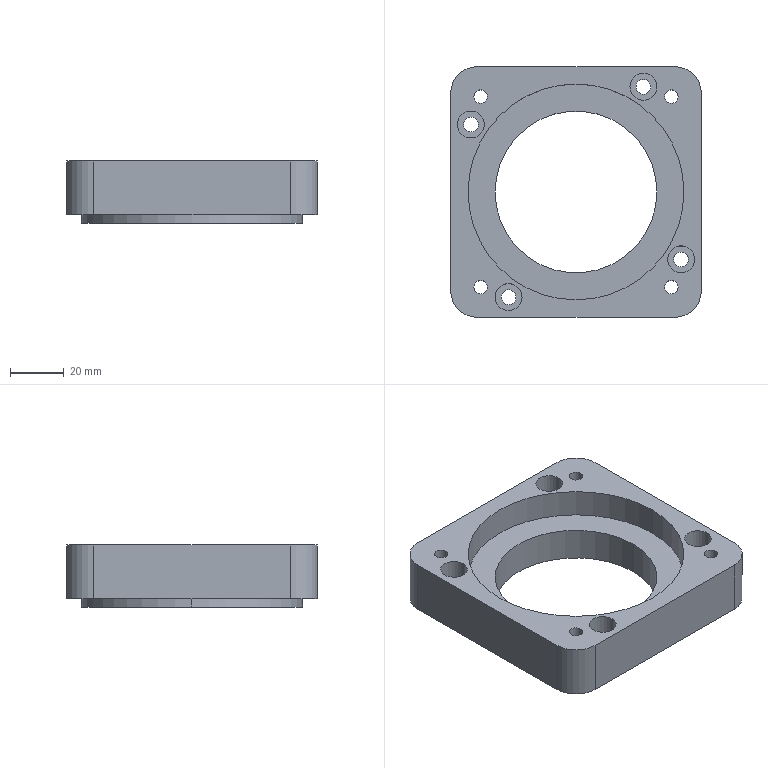Part | SolidWorks | features HoleWzd 3, CirPattern 2, ICE 2, Extrusion 1, Fillet 1 | 1 solid | 46 faces | box 93 x 93 x 23 mm | volume 93388 mm3 | cylinder 34 | plane 12 | commonest cylinder face diameters 5 x8 5.5 x8 10 x8 20 x4 60 x2 80 x2
STEP:
#1=CARTESIAN_POINT('',(-44.,25.,10.3));
#2=VERTEX_POINT('',#1);
#3=CARTESIAN_POINT('',(-34.,25.,10.3));
#4=VERTEX_POINT('',#3);
#5=CARTESIAN_POINT('',(-39.,25.,10.3));
#6=DIRECTION('',(0.,0.,1.));
#7=DIRECTION('',(1.,0.,0.));
#8=AXIS2_PLACEMENT_3D('',#5,#6,#7);
#9=CIRCLE('',#8,5.);
#10=EDGE_CURVE('',#2,#4,#9,.T.);
#11=ORIENTED_EDGE('',*,*,#10,.F.);
#12=CARTESIAN_POINT('',(-44.,25.,20.));
#13=VERTEX_POINT('',#12);
#14=CARTESIAN_POINT('',(-44.,25.,20.));
#15=DIRECTION('',(0.,0.,1.));
#16=VECTOR('',#15,1000.);
#17=LINE('',#14,#16);
#18=EDGE_CURVE('',#2,#13,#17,.T.);
#19=ORIENTED_EDGE('',*,*,#18,.T.);
#20=CARTESIAN_POINT('',(-34.,25.,20.));
#21=VERTEX_POINT('',#20);
#22=CARTESIAN_POINT('',(-39.,25.,20.));
#23=DIRECTION('',(0.,0.,1.));
#24=DIRECTION('',(1.,0.,0.));
#25=AXIS2_PLACEMENT_3D('',#22,#23,#24);
#26=CIRCLE('',#25,5.);
#27=EDGE_CURVE('',#13,#21,#26,.T.);
#28=ORIENTED_EDGE('',*,*,#27,.T.);
#29=CARTESIAN_POINT('',(-34.,25.,20.));
#30=DIRECTION('',(0.,0.,1.));
#31=VECTOR('',#30,1000.);
#32=LINE('',#29,#31);
#33=EDGE_CURVE('',#4,#21,#32,.T.);
#34=ORIENTED_EDGE('',*,*,#33,.F.);
#35=EDGE_LOOP('',(#11,#19,#28,#34));
#36=FACE_OUTER_BOUND('',#35,.T.);
#37=CARTESIAN_POINT('',(-39.,25.,20.));
#38=DIRECTION('',(0.,0.,1.));
#39=DIRECTION('',(1.,0.,0.));
#40=AXIS2_PLACEMENT_3D('',#37,#38,#39);
#41=CYLINDRICAL_SURFACE('',#40,5.);
#42=ADVANCED_FACE('',(#36),#41,.F.);
#43=CARTESIAN_POINT('',(-36.25,25.,0.));
#44=VERTEX_POINT('',#43);
#45=CARTESIAN_POINT('',(-41.75,25.,0.));
#46=VERTEX_POINT('',#45);
#47=CARTESIAN_POINT('',(-39.,25.,0.));
#48=DIRECTION('',(0.,0.,-1.));
#49=DIRECTION('',(-1.,0.,0.));
#50=AXIS2_PLACEMENT_3D('',#47,#48,#49);
#51=CIRCLE('',#50,2.75);
#52=EDGE_CURVE('',#44,#46,#51,.T.);
#53=ORIENTED_EDGE('',*,*,#52,.T.);
#54=CARTESIAN_POINT('',(-41.75,25.,10.3));
#55=VERTEX_POINT('',#54);
#56=CARTESIAN_POINT('',(-41.75,25.,20.));
#57=DIRECTION('',(0.,0.,1.));
#58=VECTOR('',#57,1000.);
#59=LINE('',#56,#58);
#60=EDGE_CURVE('',#46,#55,#59,.T.);
#61=ORIENTED_EDGE('',*,*,#60,.T.);
#62=CARTESIAN_POINT('',(-36.25,25.,10.3));
#63=VERTEX_POINT('',#62);
#64=CARTESIAN_POINT('',(-39.,25.,10.3));
#65=DIRECTION('',(0.,0.,1.));
#66=DIRECTION('',(1.,0.,0.));
#67=AXIS2_PLACEMENT_3D('',#64,#65,#66);
#68=CIRCLE('',#67,2.75);
#69=EDGE_CURVE('',#55,#63,#68,.T.);
#70=ORIENTED_EDGE('',*,*,#69,.T.);
#71=CARTESIAN_POINT('',(-36.25,25.,20.));
#72=DIRECTION('',(0.,0.,1.));
#73=VECTOR('',#72,1000.);
#74=LINE('',#71,#73);
#75=EDGE_CURVE('',#44,#63,#74,.T.);
#76=ORIENTED_EDGE('',*,*,#75,.F.);
#77=EDGE_LOOP('',(#53,#61,#70,#76));
#78=FACE_OUTER_BOUND('',#77,.T.);
#79=CARTESIAN_POINT('',(-39.,25.,20.));
#80=DIRECTION('',(0.,0.,1.));
#81=DIRECTION('',(1.,0.,0.));
#82=AXIS2_PLACEMENT_3D('',#79,#80,#81);
#83=CYLINDRICAL_SURFACE('',#82,2.75);
#84=ADVANCED_FACE('',(#78),#83,.F.);
#85=CARTESIAN_POINT('',(20.,39.,10.3));
#86=VERTEX_POINT('',#85);
#87=CARTESIAN_POINT('',(30.,39.,10.3));
#88=VERTEX_POINT('',#87);
#89=CARTESIAN_POINT('',(25.,39.,10.3));
#90=DIRECTION('',(0.,0.,1.));
#91=DIRECTION('',(1.,0.,0.));
#92=AXIS2_PLACEMENT_3D('',#89,#90,#91);
#93=CIRCLE('',#92,5.);
#94=EDGE_CURVE('',#86,#88,#93,.T.);
#95=ORIENTED_EDGE('',*,*,#94,.F.);
#96=CARTESIAN_POINT('',(20.,39.,20.));
#97=VERTEX_POINT('',#96);
#98=CARTESIAN_POINT('',(20.,39.,20.));
#99=DIRECTION('',(0.,0.,1.));
#100=VECTOR('',#99,1000.);
#101=LINE('',#98,#100);
#102=EDGE_CURVE('',#86,#97,#101,.T.);
#103=ORIENTED_EDGE('',*,*,#102,.T.);
#104=CARTESIAN_POINT('',(30.,39.,20.));
#105=VERTEX_POINT('',#104);
#106=CARTESIAN_POINT('',(25.,39.,20.));
#107=DIRECTION('',(0.,0.,1.));
#108=DIRECTION('',(1.,0.,0.));
#109=AXIS2_PLACEMENT_3D('',#106,#107,#108);
#110=CIRCLE('',#109,5.);
#111=EDGE_CURVE('',#97,#105,#110,.T.);
#112=ORIENTED_EDGE('',*,*,#111,.T.);
#113=CARTESIAN_POINT('',(30.,39.,20.));
#114=DIRECTION('',(0.,0.,1.));
#115=VECTOR('',#114,1000.);
#116=LINE('',#113,#115);
#117=EDGE_CURVE('',#88,#105,#116,.T.);
#118=ORIENTED_EDGE('',*,*,#117,.F.);
#119=EDGE_LOOP('',(#95,#103,#112,#118));
#120=FACE_OUTER_BOUND('',#119,.T.);
#121=CARTESIAN_POINT('',(25.,39.,20.));
#122=DIRECTION('',(0.,0.,1.));
#123=DIRECTION('',(1.,0.,0.));
#124=AXIS2_PLACEMENT_3D('',#121,#122,#123);
#125=CYLINDRICAL_SURFACE('',#124,5.);
#126=ADVANCED_FACE('',(#120),#125,.F.);
#127=CARTESIAN_POINT('',(27.75,39.,0.));
#128=VERTEX_POINT('',#127);
#129=CARTESIAN_POINT('',(22.25,39.,0.));
#130=VERTEX_POINT('',#129);
#131=CARTESIAN_POINT('',(25.,39.,0.));
#132=DIRECTION('',(0.,0.,-1.));
#133=DIRECTION('',(-1.,0.,0.));
#134=AXIS2_PLACEMENT_3D('',#131,#132,#133);
#135=CIRCLE('',#134,2.75);
#136=EDGE_CURVE('',#128,#130,#135,.T.);
#137=ORIENTED_EDGE('',*,*,#136,.T.);
#138=CARTESIAN_POINT('',(22.25,39.,10.3));
#139=VERTEX_POINT('',#138);
#140=CARTESIAN_POINT('',(22.25,39.,20.));
#141=DIRECTION('',(0.,0.,1.));
#142=VECTOR('',#141,1000.);
#143=LINE('',#140,#142);
#144=EDGE_CURVE('',#130,#139,#143,.T.);
#145=ORIENTED_EDGE('',*,*,#144,.T.);
#146=CARTESIAN_POINT('',(27.75,39.,10.3));
#147=VERTEX_POINT('',#146);
#148=CARTESIAN_POINT('',(25.,39.,10.3));
#149=DIRECTION('',(0.,0.,1.));
#150=DIRECTION('',(1.,0.,0.));
#151=AXIS2_PLACEMENT_3D('',#148,#149,#150);
#152=CIRCLE('',#151,2.75);
#153=EDGE_CURVE('',#139,#147,#152,.T.);
#154=ORIENTED_EDGE('',*,*,#153,.T.);
#155=CARTESIAN_POINT('',(27.75,39.,20.));
#156=DIRECTION('',(0.,0.,1.));
#157=VECTOR('',#156,1000.);
#158=LINE('',#155,#157);
#159=EDGE_CURVE('',#128,#147,#158,.T.);
#160=ORIENTED_EDGE('',*,*,#159,.F.);
#161=EDGE_LOOP('',(#137,#145,#154,#160));
#162=FACE_OUTER_BOUND('',#161,.T.);
#163=CARTESIAN_POINT('',(25.,39.,20.));
#164=DIRECTION('',(0.,0.,1.));
#165=DIRECTION('',(1.,0.,0.));
#166=AXIS2_PLACEMENT_3D('',#163,#164,#165);
#167=CYLINDRICAL_SURFACE('',#166,2.75);
#168=ADVANCED_FACE('',(#162),#167,.F.);
#169=CARTESIAN_POINT('',(34.,-25.,10.3));
#170=VERTEX_POINT('',#169);
#171=CARTESIAN_POINT('',(44.,-25.,10.3));
#172=VERTEX_POINT('',#171);
#173=CARTESIAN_POINT('',(39.,-25.,10.3));
#174=DIRECTION('',(0.,0.,1.));
#175=DIRECTION('',(1.,0.,0.));
#176=AXIS2_PLACEMENT_3D('',#173,#174,#175);
#177=CIRCLE('',#176,5.);
#178=EDGE_CURVE('',#170,#172,#177,.T.);
#179=ORIENTED_EDGE('',*,*,#178,.F.);
#180=CARTESIAN_POINT('',(34.,-25.,20.));
#181=VERTEX_POINT('',#180);
#182=CARTESIAN_POINT('',(34.,-25.,20.));
#183=DIRECTION('',(0.,0.,1.));
#184=VECTOR('',#183,1000.);
#185=LINE('',#182,#184);
#186=EDGE_CURVE('',#170,#181,#185,.T.);
#187=ORIENTED_EDGE('',*,*,#186,.T.);
#188=CARTESIAN_POINT('',(44.,-25.,20.));
#189=VERTEX_POINT('',#188);
#190=CARTESIAN_POINT('',(39.,-25.,20.));
#191=DIRECTION('',(0.,0.,1.));
#192=DIRECTION('',(1.,0.,0.));
#193=AXIS2_PLACEMENT_3D('',#190,#191,#192);
#194=CIRCLE('',#193,5.);
#195=EDGE_CURVE('',#181,#189,#194,.T.);
#196=ORIENTED_EDGE('',*,*,#195,.T.);
#197=CARTESIAN_POINT('',(44.,-25.,20.));
#198=DIRECTION('',(0.,0.,1.));
#199=VECTOR('',#198,1000.);
#200=LINE('',#197,#199);
#201=EDGE_CURVE('',#172,#189,#200,.T.);
#202=ORIENTED_EDGE('',*,*,#201,.F.);
#203=EDGE_LOOP('',(#179,#187,#196,#202));
#204=FACE_OUTER_BOUND('',#203,.T.);
#205=CARTESIAN_POINT('',(39.,-25.,20.));
#206=DIRECTION('',(0.,0.,1.));
#207=DIRECTION('',(1.,0.,0.));
#208=AXIS2_PLACEMENT_3D('',#205,#206,#207);
#209=CYLINDRICAL_SURFACE('',#208,5.);
#210=ADVANCED_FACE('',(#204),#209,.F.);
#211=CARTESIAN_POINT('',(41.75,-25.,0.));
#212=VERTEX_POINT('',#211);
#213=CARTESIAN_POINT('',(36.25,-25.,0.));
#214=VERTEX_POINT('',#213);
#215=CARTESIAN_POINT('',(39.,-25.,0.));
#216=DIRECTION('',(0.,0.,-1.));
#217=DIRECTION('',(-1.,0.,0.));
#218=AXIS2_PLACEMENT_3D('',#215,#216,#217);
#219=CIRCLE('',#218,2.75);
#220=EDGE_CURVE('',#212,#214,#219,.T.);
#221=ORIENTED_EDGE('',*,*,#220,.T.);
#222=CARTESIAN_POINT('',(36.25,-25.,10.3));
#223=VERTEX_POINT('',#222);
#224=CARTESIAN_POINT('',(36.25,-25.,20.));
#225=DIRECTION('',(0.,0.,1.));
#226=VECTOR('',#225,1000.);
#227=LINE('',#224,#226);
#228=EDGE_CURVE('',#214,#223,#227,.T.);
#229=ORIENTED_EDGE('',*,*,#228,.T.);
#230=CARTESIAN_POINT('',(41.75,-25.,10.3));
#231=VERTEX_POINT('',#230);
#232=CARTESIAN_POINT('',(39.,-25.,10.3));
#233=DIRECTION('',(0.,0.,1.));
#234=DIRECTION('',(1.,0.,0.));
#235=AXIS2_PLACEMENT_3D('',#232,#233,#234);
#236=CIRCLE('',#235,2.75);
#237=EDGE_CURVE('',#223,#231,#236,.T.);
#238=ORIENTED_EDGE('',*,*,#237,.T.);
#239=CARTESIAN_POINT('',(41.75,-25.,20.));
#240=DIRECTION('',(0.,0.,1.));
#241=VECTOR('',#240,1000.);
#242=LINE('',#239,#241);
#243=EDGE_CURVE('',#212,#231,#242,.T.);
#244=ORIENTED_EDGE('',*,*,#243,.F.);
#245=EDGE_LOOP('',(#221,#229,#238,#244));
#246=FACE_OUTER_BOUND('',#245,.T.);
#247=CARTESIAN_POINT('',(39.,-25.,20.));
#248=DIRECTION('',(0.,0.,1.));
#249=DIRECTION('',(1.,0.,0.));
#250=AXIS2_PLACEMENT_3D('',#247,#248,#249);
#251=CYLINDRICAL_SURFACE('',#250,2.75);
#252=ADVANCED_FACE('',(#246),#251,.F.);
#253=CARTESIAN_POINT('',(-30.,-39.,10.3));
#254=VERTEX_POINT('',#253);
#255=CARTESIAN_POINT('',(-20.,-39.,10.3));
#256=VERTEX_POINT('',#255);
#257=CARTESIAN_POINT('',(-25.,-39.,10.3));
#258=DIRECTION('',(0.,0.,1.));
#259=DIRECTION('',(1.,0.,0.));
#260=AXIS2_PLACEMENT_3D('',#257,#258,#259);
#261=CIRCLE('',#260,5.);
#262=EDGE_CURVE('',#254,#256,#261,.T.);
#263=ORIENTED_EDGE('',*,*,#262,.F.);
#264=CARTESIAN_POINT('',(-30.,-39.,20.));
#265=VERTEX_POINT('',#264);
#266=CARTESIAN_POINT('',(-30.,-39.,20.));
#267=DIRECTION('',(0.,0.,1.));
#268=VECTOR('',#267,1000.);
#269=LINE('',#266,#268);
#270=EDGE_CURVE('',#254,#265,#269,.T.);
#271=ORIENTED_EDGE('',*,*,#270,.T.);
#272=CARTESIAN_POINT('',(-20.,-39.,20.));
#273=VERTEX_POINT('',#272);
#274=CARTESIAN_POINT('',(-25.,-39.,20.));
#275=DIRECTION('',(0.,0.,1.));
#276=DIRECTION('',(1.,0.,0.));
#277=AXIS2_PLACEMENT_3D('',#274,#275,#276);
#278=CIRCLE('',#277,5.);
#279=EDGE_CURVE('',#265,#273,#278,.T.);
#280=ORIENTED_EDGE('',*,*,#279,.T.);
#281=CARTESIAN_POINT('',(-20.,-39.,20.));
#282=DIRECTION('',(0.,0.,1.));
#283=VECTOR('',#282,1000.);
#284=LINE('',#281,#283);
#285=EDGE_CURVE('',#256,#273,#284,.T.);
#286=ORIENTED_EDGE('',*,*,#285,.F.);
#287=EDGE_LOOP('',(#263,#271,#280,#286));
#288=FACE_OUTER_BOUND('',#287,.T.);
#289=CARTESIAN_POINT('',(-25.,-39.,20.));
#290=DIRECTION('',(0.,0.,1.));
#291=DIRECTION('',(1.,0.,0.));
#292=AXIS2_PLACEMENT_3D('',#289,#290,#291);
#293=CYLINDRICAL_SURFACE('',#292,5.);
#294=ADVANCED_FACE('',(#288),#293,.F.);
#295=CARTESIAN_POINT('',(-22.25,-39.,0.));
#296=VERTEX_POINT('',#295);
#297=CARTESIAN_POINT('',(-27.75,-39.,0.));
#298=VERTEX_POINT('',#297);
#299=CARTESIAN_POINT('',(-25.,-39.,0.));
#300=DIRECTION('',(0.,0.,-1.));
#301=DIRECTION('',(-1.,0.,0.));
#302=AXIS2_PLACEMENT_3D('',#299,#300,#301);
#303=CIRCLE('',#302,2.75);
#304=EDGE_CURVE('',#296,#298,#303,.T.);
#305=ORIENTED_EDGE('',*,*,#304,.T.);
#306=CARTESIAN_POINT('',(-27.75,-39.,10.3));
#307=VERTEX_POINT('',#306);
#308=CARTESIAN_POINT('',(-27.75,-39.,20.));
#309=DIRECTION('',(0.,0.,1.));
#310=VECTOR('',#309,1000.);
#311=LINE('',#308,#310);
#312=EDGE_CURVE('',#298,#307,#311,.T.);
#313=ORIENTED_EDGE('',*,*,#312,.T.);
#314=CARTESIAN_POINT('',(-22.25,-39.,10.3));
#315=VERTEX_POINT('',#314);
#316=CARTESIAN_POINT('',(-25.,-39.,10.3));
#317=DIRECTION('',(0.,0.,1.));
#318=DIRECTION('',(1.,0.,0.));
#319=AXIS2_PLACEMENT_3D('',#316,#317,#318);
#320=CIRCLE('',#319,2.75);
#321=EDGE_CURVE('',#307,#315,#320,.T.);
#322=ORIENTED_EDGE('',*,*,#321,.T.);
#323=CARTESIAN_POINT('',(-22.25,-39.,20.));
#324=DIRECTION('',(0.,0.,1.));
#325=VECTOR('',#324,1000.);
#326=LINE('',#323,#325);
#327=EDGE_CURVE('',#296,#315,#326,.T.);
#328=ORIENTED_EDGE('',*,*,#327,.F.);
#329=EDGE_LOOP('',(#305,#313,#322,#328));
#330=FACE_OUTER_BOUND('',#329,.T.);
#331=CARTESIAN_POINT('',(-25.,-39.,20.));
#332=DIRECTION('',(0.,0.,1.));
#333=DIRECTION('',(1.,0.,0.));
#334=AXIS2_PLACEMENT_3D('',#331,#332,#333);
#335=CYLINDRICAL_SURFACE('',#334,2.75);
#336=ADVANCED_FACE('',(#330),#335,.F.);
#337=CARTESIAN_POINT('',(-32.855,35.355,0.));
#338=VERTEX_POINT('',#337);
#339=CARTESIAN_POINT('',(-37.855,35.355,0.));
#340=VERTEX_POINT('',#339);
#341=CARTESIAN_POINT('',(-35.355,35.355,0.));
#342=DIRECTION('',(0.,0.,-1.));
#343=DIRECTION('',(-1.,0.,0.));
#344=AXIS2_PLACEMENT_3D('',#341,#342,#343);
#345=CIRCLE('',#344,2.5);
#346=EDGE_CURVE('',#338,#340,#345,.T.);
#347=ORIENTED_EDGE('',*,*,#346,.T.);
#348=CARTESIAN_POINT('',(-37.855,35.355,20.));
#349=VERTEX_POINT('',#348);
#350=CARTESIAN_POINT('',(-37.855,35.355,20.));
#351=DIRECTION('',(0.,0.,1.));
#352=VECTOR('',#351,1000.);
#353=LINE('',#350,#352);
#354=EDGE_CURVE('',#340,#349,#353,.T.);
#355=ORIENTED_EDGE('',*,*,#354,.T.);
#356=CARTESIAN_POINT('',(-32.855,35.355,20.));
#357=VERTEX_POINT('',#356);
#358=CARTESIAN_POINT('',(-35.355,35.355,20.));
#359=DIRECTION('',(0.,0.,1.));
#360=DIRECTION('',(1.,0.,0.));
#361=AXIS2_PLACEMENT_3D('',#358,#359,#360);
#362=CIRCLE('',#361,2.5);
#363=EDGE_CURVE('',#349,#357,#362,.T.);
#364=ORIENTED_EDGE('',*,*,#363,.T.);
#365=CARTESIAN_POINT('',(-32.855,35.355,20.));
#366=DIRECTION('',(0.,0.,1.));
#367=VECTOR('',#366,1000.);
#368=LINE('',#365,#367);
#369=EDGE_CURVE('',#338,#357,#368,.T.);
#370=ORIENTED_EDGE('',*,*,#369,.F.);
#371=EDGE_LOOP('',(#347,#355,#364,#370));
#372=FACE_OUTER_BOUND('',#371,.T.);
#373=CARTESIAN_POINT('',(-35.355,35.355,20.));
#374=DIRECTION('',(0.,0.,1.));
#375=DIRECTION('',(1.,0.,0.));
#376=AXIS2_PLACEMENT_3D('',#373,#374,#375);
#377=CYLINDRICAL_SURFACE('',#376,2.5);
#378=ADVANCED_FACE('',(#372),#377,.F.);
#379=CARTESIAN_POINT('',(37.855,35.355,0.));
#380=VERTEX_POINT('',#379);
#381=CARTESIAN_POINT('',(32.855,35.355,0.));
#382=VERTEX_POINT('',#381);
#383=CARTESIAN_POINT('',(35.355,35.355,0.));
#384=DIRECTION('',(0.,0.,-1.));
#385=DIRECTION('',(-1.,0.,0.));
#386=AXIS2_PLACEMENT_3D('',#383,#384,#385);
#387=CIRCLE('',#386,2.5);
#388=EDGE_CURVE('',#380,#382,#387,.T.);
#389=ORIENTED_EDGE('',*,*,#388,.T.);
#390=CARTESIAN_POINT('',(32.855,35.355,20.));
#391=VERTEX_POINT('',#390);
#392=CARTESIAN_POINT('',(32.855,35.355,20.));
#393=DIRECTION('',(0.,0.,1.));
#394=VECTOR('',#393,1000.);
#395=LINE('',#392,#394);
#396=EDGE_CURVE('',#382,#391,#395,.T.);
#397=ORIENTED_EDGE('',*,*,#396,.T.);
#398=CARTESIAN_POINT('',(37.855,35.355,20.));
#399=VERTEX_POINT('',#398);
#400=CARTESIAN_POINT('',(35.355,35.355,20.));
#401=DIRECTION('',(0.,0.,1.));
#402=DIRECTION('',(1.,0.,0.));
#403=AXIS2_PLACEMENT_3D('',#400,#401,#402);
#404=CIRCLE('',#403,2.5);
#405=EDGE_CURVE('',#391,#399,#404,.T.);
#406=ORIENTED_EDGE('',*,*,#405,.T.);
#407=CARTESIAN_POINT('',(37.855,35.355,20.));
#408=DIRECTION('',(0.,0.,1.));
#409=VECTOR('',#408,1000.);
#410=LINE('',#407,#409);
#411=EDGE_CURVE('',#380,#399,#410,.T.);
#412=ORIENTED_EDGE('',*,*,#411,.F.);
#413=EDGE_LOOP('',(#389,#397,#406,#412));
#414=FACE_OUTER_BOUND('',#413,.T.);
#415=CARTESIAN_POINT('',(35.355,35.355,20.));
#416=DIRECTION('',(0.,0.,1.));
#417=DIRECTION('',(1.,0.,0.));
#418=AXIS2_PLACEMENT_3D('',#415,#416,#417);
#419=CYLINDRICAL_SURFACE('',#418,2.5);
#420=ADVANCED_FACE('',(#414),#419,.F.);
#421=CARTESIAN_POINT('',(37.855,-35.355,0.));
#422=VERTEX_POINT('',#421);
#423=CARTESIAN_POINT('',(32.855,-35.355,0.));
#424=VERTEX_POINT('',#423);
#425=CARTESIAN_POINT('',(35.355,-35.355,0.));
#426=DIRECTION('',(0.,0.,-1.));
#427=DIRECTION('',(-1.,0.,0.));
#428=AXIS2_PLACEMENT_3D('',#425,#426,#427);
#429=CIRCLE('',#428,2.5);
#430=EDGE_CURVE('',#422,#424,#429,.T.);
#431=ORIENTED_EDGE('',*,*,#430,.T.);
#432=CARTESIAN_POINT('',(32.855,-35.355,20.));
#433=VERTEX_POINT('',#432);
#434=CARTESIAN_POINT('',(32.855,-35.355,20.));
#435=DIRECTION('',(0.,0.,1.));
#436=VECTOR('',#435,1000.);
#437=LINE('',#434,#436);
#438=EDGE_CURVE('',#424,#433,#437,.T.);
#439=ORIENTED_EDGE('',*,*,#438,.T.);
#440=CARTESIAN_POINT('',(37.855,-35.355,20.));
#441=VERTEX_POINT('',#440);
#442=CARTESIAN_POINT('',(35.355,-35.355,20.));
#443=DIRECTION('',(0.,0.,1.));
#444=DIRECTION('',(1.,0.,0.));
#445=AXIS2_PLACEMENT_3D('',#442,#443,#444);
#446=CIRCLE('',#445,2.5);
#447=EDGE_CURVE('',#433,#441,#446,.T.);
#448=ORIENTED_EDGE('',*,*,#447,.T.);
#449=CARTESIAN_POINT('',(37.855,-35.355,20.));
#450=DIRECTION('',(0.,0.,1.));
#451=VECTOR('',#450,1000.);
#452=LINE('',#449,#451);
#453=EDGE_CURVE('',#422,#441,#452,.T.);
#454=ORIENTED_EDGE('',*,*,#453,.F.);
#455=EDGE_LOOP('',(#431,#439,#448,#454));
#456=FACE_OUTER_BOUND('',#455,.T.);
#457=CARTESIAN_POINT('',(35.355,-35.355,20.));
#458=DIRECTION('',(0.,0.,1.));
#459=DIRECTION('',(1.,0.,0.));
#460=AXIS2_PLACEMENT_3D('',#457,#458,#459);
#461=CYLINDRICAL_SURFACE('',#460,2.5);
#462=ADVANCED_FACE('',(#456),#461,.F.);
#463=CARTESIAN_POINT('',(-32.855,-35.355,0.));
#464=VERTEX_POINT('',#463);
#465=CARTESIAN_POINT('',(-37.855,-35.355,0.));
#466=VERTEX_POINT('',#465);
#467=CARTESIAN_POINT('',(-35.355,-35.355,0.));
#468=DIRECTION('',(0.,0.,-1.));
#469=DIRECTION('',(-1.,0.,0.));
#470=AXIS2_PLACEMENT_3D('',#467,#468,#469);
#471=CIRCLE('',#470,2.5);
#472=EDGE_CURVE('',#464,#466,#471,.T.);
#473=ORIENTED_EDGE('',*,*,#472,.T.);
#474=CARTESIAN_POINT('',(-37.855,-35.355,20.));
#475=VERTEX_POINT('',#474);
#476=CARTESIAN_POINT('',(-37.855,-35.355,20.));
#477=DIRECTION('',(0.,0.,1.));
#478=VECTOR('',#477,1000.);
#479=LINE('',#476,#478);
#480=EDGE_CURVE('',#466,#475,#479,.T.);
#481=ORIENTED_EDGE('',*,*,#480,.T.);
#482=CARTESIAN_POINT('',(-32.855,-35.355,20.));
#483=VERTEX_POINT('',#482);
#484=CARTESIAN_POINT('',(-35.355,-35.355,20.));
#485=DIRECTION('',(0.,0.,1.));
#486=DIRECTION('',(1.,0.,0.));
#487=AXIS2_PLACEMENT_3D('',#484,#485,#486);
#488=CIRCLE('',#487,2.5);
#489=EDGE_CURVE('',#475,#483,#488,.T.);
#490=ORIENTED_EDGE('',*,*,#489,.T.);
#491=CARTESIAN_POINT('',(-32.855,-35.355,20.));
#492=DIRECTION('',(0.,0.,1.));
#493=VECTOR('',#492,1000.);
#494=LINE('',#491,#493);
#495=EDGE_CURVE('',#464,#483,#494,.T.);
#496=ORIENTED_EDGE('',*,*,#495,.F.);
#497=EDGE_LOOP('',(#473,#481,#490,#496));
#498=FACE_OUTER_BOUND('',#497,.T.);
#499=CARTESIAN_POINT('',(-35.355,-35.355,20.));
#500=DIRECTION('',(0.,0.,1.));
#501=DIRECTION('',(1.,0.,0.));
#502=AXIS2_PLACEMENT_3D('',#499,#500,#501);
#503=CYLINDRICAL_SURFACE('',#502,2.5);
#504=ADVANCED_FACE('',(#498),#503,.F.);
#505=CARTESIAN_POINT('',(-40.,0.,9.5));
#506=VERTEX_POINT('',#505);
#507=CARTESIAN_POINT('',(40.,0.,9.5));
#508=VERTEX_POINT('',#507);
#509=CARTESIAN_POINT('',(0.,0.,9.5));
#510=DIRECTION('',(0.,0.,1.));
#511=DIRECTION('',(1.,0.,0.));
#512=AXIS2_PLACEMENT_3D('',#509,#510,#511);
#513=CIRCLE('',#512,40.);
#514=EDGE_CURVE('',#506,#508,#513,.T.);
#515=ORIENTED_EDGE('',*,*,#514,.F.);
#516=CARTESIAN_POINT('',(-40.,0.,20.));
#517=VERTEX_POINT('',#516);
#518=CARTESIAN_POINT('',(-40.,0.,9.5));
#519=DIRECTION('',(0.,0.,1.));
#520=VECTOR('',#519,1000.);
#521=LINE('',#518,#520);
#522=EDGE_CURVE('',#506,#517,#521,.T.);
#523=ORIENTED_EDGE('',*,*,#522,.T.);
#524=CARTESIAN_POINT('',(40.,0.,20.));
#525=VERTEX_POINT('',#524);
#526=CARTESIAN_POINT('',(0.,0.,20.));
#527=DIRECTION('',(0.,0.,1.));
#528=DIRECTION('',(1.,0.,0.));
#529=AXIS2_PLACEMENT_3D('',#526,#527,#528);
#530=CIRCLE('',#529,40.);
#531=EDGE_CURVE('',#517,#525,#530,.T.);
#532=ORIENTED_EDGE('',*,*,#531,.T.);
#533=CARTESIAN_POINT('',(40.,0.,9.5));
#534=DIRECTION('',(0.,0.,1.));
#535=VECTOR('',#534,1000.);
#536=LINE('',#533,#535);
#537=EDGE_CURVE('',#508,#525,#536,.T.);
#538=ORIENTED_EDGE('',*,*,#537,.F.);
#539=EDGE_LOOP('',(#515,#523,#532,#538));
#540=FACE_OUTER_BOUND('',#539,.T.);
#541=CARTESIAN_POINT('',(0.,0.,9.5));
#542=DIRECTION('',(0.,0.,1.));
#543=DIRECTION('',(1.,0.,0.));
#544=AXIS2_PLACEMENT_3D('',#541,#542,#543);
#545=CYLINDRICAL_SURFACE('',#544,40.);
#546=ADVANCED_FACE('',(#540),#545,.F.);
#547=CARTESIAN_POINT('',(-41.,0.,-3.));
#548=VERTEX_POINT('',#547);
#549=CARTESIAN_POINT('',(41.,0.,-3.));
#550=VERTEX_POINT('',#549);
#551=CARTESIAN_POINT('',(0.,0.,-3.));
#552=DIRECTION('',(0.,0.,-1.));
#553=DIRECTION('',(-1.,0.,0.));
#554=AXIS2_PLACEMENT_3D('',#551,#552,#553);
#555=CIRCLE('',#554,41.);
#556=EDGE_CURVE('',#548,#550,#555,.T.);
#557=ORIENTED_EDGE('',*,*,#556,.F.);
#558=CARTESIAN_POINT('',(-41.,0.,0.));
#559=VERTEX_POINT('',#558);
#560=CARTESIAN_POINT('',(-41.,0.,-3.));
#561=DIRECTION('',(0.,0.,1.));
#562=VECTOR('',#561,1000.);
#563=LINE('',#560,#562);
#564=EDGE_CURVE('',#548,#559,#563,.T.);
#565=ORIENTED_EDGE('',*,*,#564,.T.);
#566=CARTESIAN_POINT('',(41.,0.,0.));
#567=VERTEX_POINT('',#566);
#568=CARTESIAN_POINT('',(0.,0.,0.));
#569=DIRECTION('',(0.,0.,-1.));
#570=DIRECTION('',(-1.,0.,0.));
#571=AXIS2_PLACEMENT_3D('',#568,#569,#570);
#572=CIRCLE('',#571,41.);
#573=EDGE_CURVE('',#559,#567,#572,.T.);
#574=ORIENTED_EDGE('',*,*,#573,.T.);
#575=CARTESIAN_POINT('',(41.,0.,-3.));
#576=DIRECTION('',(0.,0.,1.));
#577=VECTOR('',#576,1000.);
#578=LINE('',#575,#577);
#579=EDGE_CURVE('',#550,#567,#578,.T.);
#580=ORIENTED_EDGE('',*,*,#579,.F.);
#581=EDGE_LOOP('',(#557,#565,#574,#580));
#582=FACE_OUTER_BOUND('',#581,.T.);
#583=CARTESIAN_POINT('',(0.,0.,-3.));
#584=DIRECTION('',(0.,0.,1.));
#585=DIRECTION('',(1.,0.,0.));
#586=AXIS2_PLACEMENT_3D('',#583,#584,#585);
#587=CYLINDRICAL_SURFACE('',#586,41.);
#588=ADVANCED_FACE('',(#582),#587,.T.);
#589=CARTESIAN_POINT('',(-30.,0.,9.5));
#590=VERTEX_POINT('',#589);
#591=CARTESIAN_POINT('',(30.,0.,9.5));
#592=VERTEX_POINT('',#591);
#593=CARTESIAN_POINT('',(0.,0.,9.5));
#594=DIRECTION('',(0.,0.,1.));
#595=DIRECTION('',(1.,0.,0.));
#596=AXIS2_PLACEMENT_3D('',#593,#594,#595);
#597=CIRCLE('',#596,30.);
#598=EDGE_CURVE('',#590,#592,#597,.T.);
#599=ORIENTED_EDGE('',*,*,#598,.T.);
#600=CARTESIAN_POINT('',(30.,0.,-3.));
#601=VERTEX_POINT('',#600);
#602=CARTESIAN_POINT('',(30.,0.,20.));
#603=DIRECTION('',(0.,0.,-1.));
#604=VECTOR('',#603,1000.);
#605=LINE('',#602,#604);
#606=EDGE_CURVE('',#592,#601,#605,.T.);
#607=ORIENTED_EDGE('',*,*,#606,.T.);
#608=CARTESIAN_POINT('',(-30.,0.,-3.));
#609=VERTEX_POINT('',#608);
#610=CARTESIAN_POINT('',(0.,0.,-3.));
#611=DIRECTION('',(0.,0.,-1.));
#612=DIRECTION('',(-1.,0.,0.));
#613=AXIS2_PLACEMENT_3D('',#610,#611,#612);
#614=CIRCLE('',#613,30.);
#615=EDGE_CURVE('',#601,#609,#614,.T.);
#616=ORIENTED_EDGE('',*,*,#615,.T.);
#617=CARTESIAN_POINT('',(-30.,0.,20.));
#618=DIRECTION('',(0.,0.,-1.));
#619=VECTOR('',#618,1000.);
#620=LINE('',#617,#619);
#621=EDGE_CURVE('',#590,#609,#620,.T.);
#622=ORIENTED_EDGE('',*,*,#621,.F.);
#623=EDGE_LOOP('',(#599,#607,#616,#622));
#624=FACE_OUTER_BOUND('',#623,.T.);
#625=CARTESIAN_POINT('',(0.,0.,20.));
#626=DIRECTION('',(0.,0.,-1.));
#627=DIRECTION('',(-1.,0.,0.));
#628=AXIS2_PLACEMENT_3D('',#625,#626,#627);
#629=CYLINDRICAL_SURFACE('',#628,30.);
#630=ADVANCED_FACE('',(#624),#629,.F.);
#631=CARTESIAN_POINT('',(25.,39.,20.));
#632=DIRECTION('',(0.,0.,1.));
#633=DIRECTION('',(1.,0.,0.));
#634=AXIS2_PLACEMENT_3D('',#631,#632,#633);
#635=CIRCLE('',#634,5.);
#636=EDGE_CURVE('',#105,#97,#635,.T.);
#637=ORIENTED_EDGE('',*,*,#636,.F.);
#638=ORIENTED_EDGE('',*,*,#111,.F.);
#639=EDGE_LOOP('',(#637,#638));
#640=FACE_BOUND('',#639,.T.);
#641=CARTESIAN_POINT('',(39.,-25.,20.));
#642=DIRECTION('',(0.,0.,1.));
#643=DIRECTION('',(1.,0.,0.));
#644=AXIS2_PLACEMENT_3D('',#641,#642,#643);
#645=CIRCLE('',#644,5.);
#646=EDGE_CURVE('',#189,#181,#645,.T.);
#647=ORIENTED_EDGE('',*,*,#646,.F.);
#648=ORIENTED_EDGE('',*,*,#195,.F.);
#649=EDGE_LOOP('',(#647,#648));
#650=FACE_BOUND('',#649,.T.);
#651=CARTESIAN_POINT('',(-25.,-39.,20.));
#652=DIRECTION('',(0.,0.,1.));
#653=DIRECTION('',(1.,0.,0.));
#654=AXIS2_PLACEMENT_3D('',#651,#652,#653);
#655=CIRCLE('',#654,5.);
#656=EDGE_CURVE('',#273,#265,#655,.T.);
#657=ORIENTED_EDGE('',*,*,#656,.F.);
#658=ORIENTED_EDGE('',*,*,#279,.F.);
#659=EDGE_LOOP('',(#657,#658));
#660=FACE_BOUND('',#659,.T.);
#661=CARTESIAN_POINT('',(-35.355,35.355,20.));
#662=DIRECTION('',(0.,0.,1.));
#663=DIRECTION('',(1.,0.,0.));
#664=AXIS2_PLACEMENT_3D('',#661,#662,#663);
#665=CIRCLE('',#664,2.5);
#666=EDGE_CURVE('',#357,#349,#665,.T.);
#667=ORIENTED_EDGE('',*,*,#666,.F.);
#668=ORIENTED_EDGE('',*,*,#363,.F.);
#669=EDGE_LOOP('',(#667,#668));
#670=FACE_BOUND('',#669,.T.);
#671=CARTESIAN_POINT('',(35.355,35.355,20.));
#672=DIRECTION('',(0.,0.,1.));
#673=DIRECTION('',(1.,0.,0.));
#674=AXIS2_PLACEMENT_3D('',#671,#672,#673);
#675=CIRCLE('',#674,2.5);
#676=EDGE_CURVE('',#399,#391,#675,.T.);
#677=ORIENTED_EDGE('',*,*,#676,.F.);
#678=ORIENTED_EDGE('',*,*,#405,.F.);
#679=EDGE_LOOP('',(#677,#678));
#680=FACE_BOUND('',#679,.T.);
#681=CARTESIAN_POINT('',(35.355,-35.355,20.));
#682=DIRECTION('',(0.,0.,1.));
#683=DIRECTION('',(1.,0.,0.));
#684=AXIS2_PLACEMENT_3D('',#681,#682,#683);
#685=CIRCLE('',#684,2.5);
#686=EDGE_CURVE('',#441,#433,#685,.T.);
#687=ORIENTED_EDGE('',*,*,#686,.F.);
#688=ORIENTED_EDGE('',*,*,#447,.F.);
#689=EDGE_LOOP('',(#687,#688));
#690=FACE_BOUND('',#689,.T.);
#691=CARTESIAN_POINT('',(-35.355,-35.355,20.));
#692=DIRECTION('',(0.,0.,1.));
#693=DIRECTION('',(1.,0.,0.));
#694=AXIS2_PLACEMENT_3D('',#691,#692,#693);
#695=CIRCLE('',#694,2.5);
#696=EDGE_CURVE('',#483,#475,#695,.T.);
#697=ORIENTED_EDGE('',*,*,#696,.F.);
#698=ORIENTED_EDGE('',*,*,#489,.F.);
#699=EDGE_LOOP('',(#697,#698));
#700=FACE_BOUND('',#699,.T.);
#701=CARTESIAN_POINT('',(0.,0.,20.));
#702=DIRECTION('',(0.,0.,1.));
#703=DIRECTION('',(1.,0.,0.));
#704=AXIS2_PLACEMENT_3D('',#701,#702,#703);
#705=CIRCLE('',#704,40.);
#706=EDGE_CURVE('',#525,#517,#705,.T.);
#707=ORIENTED_EDGE('',*,*,#706,.F.);
#708=ORIENTED_EDGE('',*,*,#531,.F.);
#709=EDGE_LOOP('',(#707,#708));
#710=FACE_BOUND('',#709,.T.);
#711=CARTESIAN_POINT('',(-46.5,36.5,20.));
#712=VERTEX_POINT('',#711);
#713=CARTESIAN_POINT('',(-46.5,-36.5,20.));
#714=VERTEX_POINT('',#713);
#715=CARTESIAN_POINT('',(-46.5,-46.5,20.));
#716=DIRECTION('',(0.,-1.,0.));
#717=VECTOR('',#716,1000.);
#718=LINE('',#715,#717);
#719=EDGE_CURVE('',#712,#714,#718,.T.);
#720=ORIENTED_EDGE('',*,*,#719,.T.);
#721=CARTESIAN_POINT('',(-36.5,-46.5,20.));
#722=VERTEX_POINT('',#721);
#723=CARTESIAN_POINT('',(-36.5,-36.5,20.));
#724=DIRECTION('',(0.,0.,1.));
#725=DIRECTION('',(-1.,0.,0.));
#726=AXIS2_PLACEMENT_3D('',#723,#724,#725);
#727=CIRCLE('',#726,10.);
#728=EDGE_CURVE('',#714,#722,#727,.T.);
#729=ORIENTED_EDGE('',*,*,#728,.T.);
#730=CARTESIAN_POINT('',(36.5,-46.5,20.));
#731=VERTEX_POINT('',#730);
#732=CARTESIAN_POINT('',(-46.5,-46.5,20.));
#733=DIRECTION('',(1.,0.,0.));
#734=VECTOR('',#733,1000.);
#735=LINE('',#732,#734);
#736=EDGE_CURVE('',#722,#731,#735,.T.);
#737=ORIENTED_EDGE('',*,*,#736,.T.);
#738=CARTESIAN_POINT('',(46.5,-36.5,20.));
#739=VERTEX_POINT('',#738);
#740=CARTESIAN_POINT('',(36.5,-36.5,20.));
#741=DIRECTION('',(0.,0.,1.));
#742=DIRECTION('',(-1.,0.,0.));
#743=AXIS2_PLACEMENT_3D('',#740,#741,#742);
#744=CIRCLE('',#743,10.);
#745=EDGE_CURVE('',#731,#739,#744,.T.);
#746=ORIENTED_EDGE('',*,*,#745,.T.);
#747=CARTESIAN_POINT('',(46.5,36.5,20.));
#748=VERTEX_POINT('',#747);
#749=CARTESIAN_POINT('',(46.5,-46.5,20.));
#750=DIRECTION('',(0.,1.,0.));
#751=VECTOR('',#750,1000.);
#752=LINE('',#749,#751);
#753=EDGE_CURVE('',#739,#748,#752,.T.);
#754=ORIENTED_EDGE('',*,*,#753,.T.);
#755=CARTESIAN_POINT('',(36.5,46.5,20.));
#756=VERTEX_POINT('',#755);
#757=CARTESIAN_POINT('',(36.5,36.5,20.));
#758=DIRECTION('',(0.,0.,1.));
#759=DIRECTION('',(-1.,0.,0.));
#760=AXIS2_PLACEMENT_3D('',#757,#758,#759);
#761=CIRCLE('',#760,10.);
#762=EDGE_CURVE('',#748,#756,#761,.T.);
#763=ORIENTED_EDGE('',*,*,#762,.T.);
#764=CARTESIAN_POINT('',(-36.5,46.5,20.));
#765=VERTEX_POINT('',#764);
#766=CARTESIAN_POINT('',(-46.5,46.5,20.));
#767=DIRECTION('',(-1.,0.,0.));
#768=VECTOR('',#767,1000.);
#769=LINE('',#766,#768);
#770=EDGE_CURVE('',#756,#765,#769,.T.);
#771=ORIENTED_EDGE('',*,*,#770,.T.);
#772=CARTESIAN_POINT('',(-36.5,36.5,20.));
#773=DIRECTION('',(0.,0.,1.));
#774=DIRECTION('',(-1.,0.,0.));
#775=AXIS2_PLACEMENT_3D('',#772,#773,#774);
#776=CIRCLE('',#775,10.);
#777=EDGE_CURVE('',#765,#712,#776,.T.);
#778=ORIENTED_EDGE('',*,*,#777,.T.);
#779=EDGE_LOOP('',(#720,#729,#737,#746,#754,#763,#771,#778));
#780=FACE_OUTER_BOUND('',#779,.T.);
#781=CARTESIAN_POINT('',(-39.,25.,20.));
#782=DIRECTION('',(0.,0.,1.));
#783=DIRECTION('',(1.,0.,0.));
#784=AXIS2_PLACEMENT_3D('',#781,#782,#783);
#785=CIRCLE('',#784,5.);
#786=EDGE_CURVE('',#21,#13,#785,.T.);
#787=ORIENTED_EDGE('',*,*,#786,.F.);
#788=ORIENTED_EDGE('',*,*,#27,.F.);
#789=EDGE_LOOP('',(#787,#788));
#790=FACE_BOUND('',#789,.T.);
#791=CARTESIAN_POINT('',(0.,0.,20.));
#792=DIRECTION('',(0.,0.,-1.));
#793=DIRECTION('',(-1.,0.,0.));
#794=AXIS2_PLACEMENT_3D('',#791,#792,#793);
#795=PLANE('',#794);
#796=ADVANCED_FACE('',(#640,#650,#660,#670,#680,#690,#700,#710,#780,#790),#795,.F.);
#797=ORIENTED_EDGE('',*,*,#606,.F.);
#798=CARTESIAN_POINT('',(0.,0.,9.5));
#799=DIRECTION('',(0.,0.,1.));
#800=DIRECTION('',(1.,0.,0.));
#801=AXIS2_PLACEMENT_3D('',#798,#799,#800);
#802=CIRCLE('',#801,30.);
#803=EDGE_CURVE('',#592,#590,#802,.T.);
#804=ORIENTED_EDGE('',*,*,#803,.T.);
#805=ORIENTED_EDGE('',*,*,#621,.T.);
#806=CARTESIAN_POINT('',(0.,0.,-3.));
#807=DIRECTION('',(0.,0.,-1.));
#808=DIRECTION('',(-1.,0.,0.));
#809=AXIS2_PLACEMENT_3D('',#806,#807,#808);
#810=CIRCLE('',#809,30.);
#811=EDGE_CURVE('',#609,#601,#810,.T.);
#812=ORIENTED_EDGE('',*,*,#811,.T.);
#813=EDGE_LOOP('',(#797,#804,#805,#812));
#814=FACE_OUTER_BOUND('',#813,.T.);
#815=CARTESIAN_POINT('',(0.,0.,20.));
#816=DIRECTION('',(0.,0.,-1.));
#817=DIRECTION('',(-1.,0.,0.));
#818=AXIS2_PLACEMENT_3D('',#815,#816,#817);
#819=CYLINDRICAL_SURFACE('',#818,30.);
#820=ADVANCED_FACE('',(#814),#819,.F.);
#821=ORIENTED_EDGE('',*,*,#52,.F.);
#822=CARTESIAN_POINT('',(-39.,25.,0.));
#823=DIRECTION('',(0.,0.,-1.));
#824=DIRECTION('',(-1.,0.,0.));
#825=AXIS2_PLACEMENT_3D('',#822,#823,#824);
#826=CIRCLE('',#825,2.75);
#827=EDGE_CURVE('',#46,#44,#826,.T.);
#828=ORIENTED_EDGE('',*,*,#827,.F.);
#829=EDGE_LOOP('',(#821,#828));
#830=FACE_BOUND('',#829,.T.);
#831=ORIENTED_EDGE('',*,*,#136,.F.);
#832=CARTESIAN_POINT('',(25.,39.,0.));
#833=DIRECTION('',(0.,0.,-1.));
#834=DIRECTION('',(-1.,0.,0.));
#835=AXIS2_PLACEMENT_3D('',#832,#833,#834);
#836=CIRCLE('',#835,2.75);
#837=EDGE_CURVE('',#130,#128,#836,.T.);
#838=ORIENTED_EDGE('',*,*,#837,.F.);
#839=EDGE_LOOP('',(#831,#838));
#840=FACE_BOUND('',#839,.T.);
#841=ORIENTED_EDGE('',*,*,#220,.F.);
#842=CARTESIAN_POINT('',(39.,-25.,0.));
#843=DIRECTION('',(0.,0.,-1.));
#844=DIRECTION('',(-1.,0.,0.));
#845=AXIS2_PLACEMENT_3D('',#842,#843,#844);
#846=CIRCLE('',#845,2.75);
#847=EDGE_CURVE('',#214,#212,#846,.T.);
#848=ORIENTED_EDGE('',*,*,#847,.F.);
#849=EDGE_LOOP('',(#841,#848));
#850=FACE_BOUND('',#849,.T.);
#851=ORIENTED_EDGE('',*,*,#304,.F.);
#852=CARTESIAN_POINT('',(-25.,-39.,0.));
#853=DIRECTION('',(0.,0.,-1.));
#854=DIRECTION('',(-1.,0.,0.));
#855=AXIS2_PLACEMENT_3D('',#852,#853,#854);
#856=CIRCLE('',#855,2.75);
#857=EDGE_CURVE('',#298,#296,#856,.T.);
#858=ORIENTED_EDGE('',*,*,#857,.F.);
#859=EDGE_LOOP('',(#851,#858));
#860=FACE_BOUND('',#859,.T.);
#861=ORIENTED_EDGE('',*,*,#346,.F.);
#862=CARTESIAN_POINT('',(-35.355,35.355,0.));
#863=DIRECTION('',(0.,0.,-1.));
#864=DIRECTION('',(-1.,0.,0.));
#865=AXIS2_PLACEMENT_3D('',#862,#863,#864);
#866=CIRCLE('',#865,2.5);
#867=EDGE_CURVE('',#340,#338,#866,.T.);
#868=ORIENTED_EDGE('',*,*,#867,.F.);
#869=EDGE_LOOP('',(#861,#868));
#870=FACE_BOUND('',#869,.T.);
#871=ORIENTED_EDGE('',*,*,#388,.F.);
#872=CARTESIAN_POINT('',(35.355,35.355,0.));
#873=DIRECTION('',(0.,0.,-1.));
#874=DIRECTION('',(-1.,0.,0.));
#875=AXIS2_PLACEMENT_3D('',#872,#873,#874);
#876=CIRCLE('',#875,2.5);
#877=EDGE_CURVE('',#382,#380,#876,.T.);
#878=ORIENTED_EDGE('',*,*,#877,.F.);
#879=EDGE_LOOP('',(#871,#878));
#880=FACE_BOUND('',#879,.T.);
#881=ORIENTED_EDGE('',*,*,#430,.F.);
#882=CARTESIAN_POINT('',(35.355,-35.355,0.));
#883=DIRECTION('',(0.,0.,-1.));
#884=DIRECTION('',(-1.,0.,0.));
#885=AXIS2_PLACEMENT_3D('',#882,#883,#884);
#886=CIRCLE('',#885,2.5);
#887=EDGE_CURVE('',#424,#422,#886,.T.);
#888=ORIENTED_EDGE('',*,*,#887,.F.);
#889=EDGE_LOOP('',(#881,#888));
#890=FACE_BOUND('',#889,.T.);
#891=ORIENTED_EDGE('',*,*,#472,.F.);
#892=CARTESIAN_POINT('',(-35.355,-35.355,0.));
#893=DIRECTION('',(0.,0.,-1.));
#894=DIRECTION('',(-1.,0.,0.));
#895=AXIS2_PLACEMENT_3D('',#892,#893,#894);
#896=CIRCLE('',#895,2.5);
#897=EDGE_CURVE('',#466,#464,#896,.T.);
#898=ORIENTED_EDGE('',*,*,#897,.F.);
#899=EDGE_LOOP('',(#891,#898));
#900=FACE_BOUND('',#899,.T.);
#901=CARTESIAN_POINT('',(0.,0.,0.));
#902=DIRECTION('',(0.,0.,-1.));
#903=DIRECTION('',(-1.,0.,0.));
#904=AXIS2_PLACEMENT_3D('',#901,#902,#903);
#905=CIRCLE('',#904,41.);
#906=EDGE_CURVE('',#567,#559,#905,.T.);
#907=ORIENTED_EDGE('',*,*,#906,.F.);
#908=ORIENTED_EDGE('',*,*,#573,.F.);
#909=EDGE_LOOP('',(#907,#908));
#910=FACE_BOUND('',#909,.T.);
#911=CARTESIAN_POINT('',(-36.5,-46.5,0.));
#912=VERTEX_POINT('',#911);
#913=CARTESIAN_POINT('',(36.5,-46.5,0.));
#914=VERTEX_POINT('',#913);
#915=CARTESIAN_POINT('',(-46.5,-46.5,0.));
#916=DIRECTION('',(1.,0.,0.));
#917=VECTOR('',#916,1000.);
#918=LINE('',#915,#917);
#919=EDGE_CURVE('',#912,#914,#918,.T.);
#920=ORIENTED_EDGE('',*,*,#919,.F.);
#921=CARTESIAN_POINT('',(-46.5,-36.5,0.));
#922=VERTEX_POINT('',#921);
#923=CARTESIAN_POINT('',(-36.5,-36.5,0.));
#924=DIRECTION('',(0.,0.,-1.));
#925=DIRECTION('',(-1.,0.,0.));
#926=AXIS2_PLACEMENT_3D('',#923,#924,#925);
#927=CIRCLE('',#926,10.);
#928=EDGE_CURVE('',#912,#922,#927,.T.);
#929=ORIENTED_EDGE('',*,*,#928,.T.);
#930=CARTESIAN_POINT('',(-46.5,36.5,0.));
#931=VERTEX_POINT('',#930);
#932=CARTESIAN_POINT('',(-46.5,-46.5,0.));
#933=DIRECTION('',(0.,-1.,0.));
#934=VECTOR('',#933,1000.);
#935=LINE('',#932,#934);
#936=EDGE_CURVE('',#931,#922,#935,.T.);
#937=ORIENTED_EDGE('',*,*,#936,.F.);
#938=CARTESIAN_POINT('',(-36.5,46.5,0.));
#939=VERTEX_POINT('',#938);
#940=CARTESIAN_POINT('',(-36.5,36.5,0.));
#941=DIRECTION('',(0.,0.,-1.));
#942=DIRECTION('',(-1.,0.,0.));
#943=AXIS2_PLACEMENT_3D('',#940,#941,#942);
#944=CIRCLE('',#943,10.);
#945=EDGE_CURVE('',#931,#939,#944,.T.);
#946=ORIENTED_EDGE('',*,*,#945,.T.);
#947=CARTESIAN_POINT('',(36.5,46.5,0.));
#948=VERTEX_POINT('',#947);
#949=CARTESIAN_POINT('',(-46.5,46.5,0.));
#950=DIRECTION('',(-1.,0.,0.));
#951=VECTOR('',#950,1000.);
#952=LINE('',#949,#951);
#953=EDGE_CURVE('',#948,#939,#952,.T.);
#954=ORIENTED_EDGE('',*,*,#953,.F.);
#955=CARTESIAN_POINT('',(46.5,36.5,0.));
#956=VERTEX_POINT('',#955);
#957=CARTESIAN_POINT('',(36.5,36.5,0.));
#958=DIRECTION('',(0.,0.,-1.));
#959=DIRECTION('',(-1.,0.,0.));
#960=AXIS2_PLACEMENT_3D('',#957,#958,#959);
#961=CIRCLE('',#960,10.);
#962=EDGE_CURVE('',#948,#956,#961,.T.);
#963=ORIENTED_EDGE('',*,*,#962,.T.);
#964=CARTESIAN_POINT('',(46.5,-36.5,0.));
#965=VERTEX_POINT('',#964);
#966=CARTESIAN_POINT('',(46.5,-46.5,0.));
#967=DIRECTION('',(0.,1.,0.));
#968=VECTOR('',#967,1000.);
#969=LINE('',#966,#968);
#970=EDGE_CURVE('',#965,#956,#969,.T.);
#971=ORIENTED_EDGE('',*,*,#970,.F.);
#972=CARTESIAN_POINT('',(36.5,-36.5,0.));
#973=DIRECTION('',(0.,0.,-1.));
#974=DIRECTION('',(-1.,0.,0.));
#975=AXIS2_PLACEMENT_3D('',#972,#973,#974);
#976=CIRCLE('',#975,10.);
#977=EDGE_CURVE('',#965,#914,#976,.T.);
#978=ORIENTED_EDGE('',*,*,#977,.T.);
#979=EDGE_LOOP('',(#920,#929,#937,#946,#954,#963,#971,#978));
#980=FACE_OUTER_BOUND('',#979,.T.);
#981=CARTESIAN_POINT('',(0.,0.,0.));
#982=DIRECTION('',(0.,0.,-1.));
#983=DIRECTION('',(-1.,0.,0.));
#984=AXIS2_PLACEMENT_3D('',#981,#982,#983);
#985=PLANE('',#984);
#986=ADVANCED_FACE('',(#830,#840,#850,#860,#870,#880,#890,#900,#910,#980),#985,.T.);
#987=ORIENTED_EDGE('',*,*,#753,.F.);
#988=CARTESIAN_POINT('',(46.5,-36.5,20.));
#989=DIRECTION('',(0.,0.,-1.));
#990=VECTOR('',#989,1000.);
#991=LINE('',#988,#990);
#992=EDGE_CURVE('',#739,#965,#991,.T.);
#993=ORIENTED_EDGE('',*,*,#992,.T.);
#994=ORIENTED_EDGE('',*,*,#970,.T.);
#995=CARTESIAN_POINT('',(46.5,36.5,20.));
#996=DIRECTION('',(0.,0.,1.));
#997=VECTOR('',#996,1000.);
#998=LINE('',#995,#997);
#999=EDGE_CURVE('',#956,#748,#998,.T.);
#1000=ORIENTED_EDGE('',*,*,#999,.T.);
#1001=EDGE_LOOP('',(#987,#993,#994,#1000));
#1002=FACE_OUTER_BOUND('',#1001,.T.);
#1003=CARTESIAN_POINT('',(46.5,-46.5,20.));
#1004=DIRECTION('',(-1.,0.,0.));
#1005=DIRECTION('',(0.,0.,1.));
#1006=AXIS2_PLACEMENT_3D('',#1003,#1004,#1005);
#1007=PLANE('',#1006);
#1008=ADVANCED_FACE('',(#1002),#1007,.F.);
#1009=ORIENTED_EDGE('',*,*,#770,.F.);
#1010=CARTESIAN_POINT('',(36.5,46.5,20.));
#1011=DIRECTION('',(0.,0.,-1.));
#1012=VECTOR('',#1011,1000.);
#1013=LINE('',#1010,#1012);
#1014=EDGE_CURVE('',#756,#948,#1013,.T.);
#1015=ORIENTED_EDGE('',*,*,#1014,.T.);
#1016=ORIENTED_EDGE('',*,*,#953,.T.);
#1017=CARTESIAN_POINT('',(-36.5,46.5,20.));
#1018=DIRECTION('',(0.,0.,1.));
#1019=VECTOR('',#1018,1000.);
#1020=LINE('',#1017,#1019);
#1021=EDGE_CURVE('',#939,#765,#1020,.T.);
#1022=ORIENTED_EDGE('',*,*,#1021,.T.);
#1023=EDGE_LOOP('',(#1009,#1015,#1016,#1022));
#1024=FACE_OUTER_BOUND('',#1023,.T.);
#1025=CARTESIAN_POINT('',(-46.5,46.5,20.));
#1026=DIRECTION('',(0.,-1.,0.));
#1027=DIRECTION('',(0.,0.,-1.));
#1028=AXIS2_PLACEMENT_3D('',#1025,#1026,#1027);
#1029=PLANE('',#1028);
#1030=ADVANCED_FACE('',(#1024),#1029,.F.);
#1031=ORIENTED_EDGE('',*,*,#936,.T.);
#1032=CARTESIAN_POINT('',(-46.5,-36.5,20.));
#1033=DIRECTION('',(0.,0.,1.));
#1034=VECTOR('',#1033,1000.);
#1035=LINE('',#1032,#1034);
#1036=EDGE_CURVE('',#922,#714,#1035,.T.);
#1037=ORIENTED_EDGE('',*,*,#1036,.T.);
#1038=ORIENTED_EDGE('',*,*,#719,.F.);
#1039=CARTESIAN_POINT('',(-46.5,36.5,20.));
#1040=DIRECTION('',(0.,0.,-1.));
#1041=VECTOR('',#1040,1000.);
#1042=LINE('',#1039,#1041);
#1043=EDGE_CURVE('',#712,#931,#1042,.T.);
#1044=ORIENTED_EDGE('',*,*,#1043,.T.);
#1045=EDGE_LOOP('',(#1031,#1037,#1038,#1044));
#1046=FACE_OUTER_BOUND('',#1045,.T.);
#1047=CARTESIAN_POINT('',(-46.5,-46.5,20.));
#1048=DIRECTION('',(1.,0.,0.));
#1049=DIRECTION('',(0.,0.,-1.));
#1050=AXIS2_PLACEMENT_3D('',#1047,#1048,#1049);
#1051=PLANE('',#1050);
#1052=ADVANCED_FACE('',(#1046),#1051,.F.);
#1053=ORIENTED_EDGE('',*,*,#736,.F.);
#1054=CARTESIAN_POINT('',(-36.5,-46.5,20.));
#1055=DIRECTION('',(0.,0.,-1.));
#1056=VECTOR('',#1055,1000.);
#1057=LINE('',#1054,#1056);
#1058=EDGE_CURVE('',#722,#912,#1057,.T.);
#1059=ORIENTED_EDGE('',*,*,#1058,.T.);
#1060=ORIENTED_EDGE('',*,*,#919,.T.);
#1061=CARTESIAN_POINT('',(36.5,-46.5,20.));
#1062=DIRECTION('',(0.,0.,1.));
#1063=VECTOR('',#1062,1000.);
#1064=LINE('',#1061,#1063);
#1065=EDGE_CURVE('',#914,#731,#1064,.T.);
#1066=ORIENTED_EDGE('',*,*,#1065,.T.);
#1067=EDGE_LOOP('',(#1053,#1059,#1060,#1066));
#1068=FACE_OUTER_BOUND('',#1067,.T.);
#1069=CARTESIAN_POINT('',(-46.5,-46.5,20.));
#1070=DIRECTION('',(0.,1.,0.));
#1071=DIRECTION('',(0.,0.,1.));
#1072=AXIS2_PLACEMENT_3D('',#1069,#1070,#1071);
#1073=PLANE('',#1072);
#1074=ADVANCED_FACE('',(#1068),#1073,.F.);
#1075=ORIENTED_EDGE('',*,*,#728,.F.);
#1076=ORIENTED_EDGE('',*,*,#1036,.F.);
#1077=ORIENTED_EDGE('',*,*,#928,.F.);
#1078=ORIENTED_EDGE('',*,*,#1058,.F.);
#1079=EDGE_LOOP('',(#1075,#1076,#1077,#1078));
#1080=FACE_OUTER_BOUND('',#1079,.T.);
#1081=CARTESIAN_POINT('',(-36.5,-36.5,20.));
#1082=DIRECTION('',(0.,0.,-1.));
#1083=DIRECTION('',(-1.,0.,0.));
#1084=AXIS2_PLACEMENT_3D('',#1081,#1082,#1083);
#1085=CYLINDRICAL_SURFACE('',#1084,10.);
#1086=ADVANCED_FACE('',(#1080),#1085,.T.);
#1087=ORIENTED_EDGE('',*,*,#745,.F.);
#1088=ORIENTED_EDGE('',*,*,#1065,.F.);
#1089=ORIENTED_EDGE('',*,*,#977,.F.);
#1090=ORIENTED_EDGE('',*,*,#992,.F.);
#1091=EDGE_LOOP('',(#1087,#1088,#1089,#1090));
#1092=FACE_OUTER_BOUND('',#1091,.T.);
#1093=CARTESIAN_POINT('',(36.5,-36.5,20.));
#1094=DIRECTION('',(0.,0.,-1.));
#1095=DIRECTION('',(-1.,0.,0.));
#1096=AXIS2_PLACEMENT_3D('',#1093,#1094,#1095);
#1097=CYLINDRICAL_SURFACE('',#1096,10.);
#1098=ADVANCED_FACE('',(#1092),#1097,.T.);
#1099=ORIENTED_EDGE('',*,*,#762,.F.);
#1100=ORIENTED_EDGE('',*,*,#999,.F.);
#1101=ORIENTED_EDGE('',*,*,#962,.F.);
#1102=ORIENTED_EDGE('',*,*,#1014,.F.);
#1103=EDGE_LOOP('',(#1099,#1100,#1101,#1102));
#1104=FACE_OUTER_BOUND('',#1103,.T.);
#1105=CARTESIAN_POINT('',(36.5,36.5,20.));
#1106=DIRECTION('',(0.,0.,-1.));
#1107=DIRECTION('',(-1.,0.,0.));
#1108=AXIS2_PLACEMENT_3D('',#1105,#1106,#1107);
#1109=CYLINDRICAL_SURFACE('',#1108,10.);
#1110=ADVANCED_FACE('',(#1104),#1109,.T.);
#1111=ORIENTED_EDGE('',*,*,#777,.F.);
#1112=ORIENTED_EDGE('',*,*,#1021,.F.);
#1113=ORIENTED_EDGE('',*,*,#945,.F.);
#1114=ORIENTED_EDGE('',*,*,#1043,.F.);
#1115=EDGE_LOOP('',(#1111,#1112,#1113,#1114));
#1116=FACE_OUTER_BOUND('',#1115,.T.);
#1117=CARTESIAN_POINT('',(-36.5,36.5,20.));
#1118=DIRECTION('',(0.,0.,-1.));
#1119=DIRECTION('',(-1.,0.,0.));
#1120=AXIS2_PLACEMENT_3D('',#1117,#1118,#1119);
#1121=CYLINDRICAL_SURFACE('',#1120,10.);
#1122=ADVANCED_FACE('',(#1116),#1121,.T.);
#1123=CARTESIAN_POINT('',(0.,0.,-3.));
#1124=DIRECTION('',(0.,0.,-1.));
#1125=DIRECTION('',(-1.,0.,0.));
#1126=AXIS2_PLACEMENT_3D('',#1123,#1124,#1125);
#1127=CIRCLE('',#1126,41.);
#1128=EDGE_CURVE('',#550,#548,#1127,.T.);
#1129=ORIENTED_EDGE('',*,*,#1128,.T.);
#1130=ORIENTED_EDGE('',*,*,#556,.T.);
#1131=EDGE_LOOP('',(#1129,#1130));
#1132=FACE_OUTER_BOUND('',#1131,.T.);
#1133=ORIENTED_EDGE('',*,*,#811,.F.);
#1134=ORIENTED_EDGE('',*,*,#615,.F.);
#1135=EDGE_LOOP('',(#1133,#1134));
#1136=FACE_BOUND('',#1135,.T.);
#1137=CARTESIAN_POINT('',(0.,0.,-3.));
#1138=DIRECTION('',(0.,0.,-1.));
#1139=DIRECTION('',(-1.,0.,0.));
#1140=AXIS2_PLACEMENT_3D('',#1137,#1138,#1139);
#1141=PLANE('',#1140);
#1142=ADVANCED_FACE('',(#1132,#1136),#1141,.T.);
#1143=ORIENTED_EDGE('',*,*,#564,.F.);
#1144=ORIENTED_EDGE('',*,*,#1128,.F.);
#1145=ORIENTED_EDGE('',*,*,#579,.T.);
#1146=ORIENTED_EDGE('',*,*,#906,.T.);
#1147=EDGE_LOOP('',(#1143,#1144,#1145,#1146));
#1148=FACE_OUTER_BOUND('',#1147,.T.);
#1149=CARTESIAN_POINT('',(0.,0.,-3.));
#1150=DIRECTION('',(0.,0.,1.));
#1151=DIRECTION('',(1.,0.,0.));
#1152=AXIS2_PLACEMENT_3D('',#1149,#1150,#1151);
#1153=CYLINDRICAL_SURFACE('',#1152,41.);
#1154=ADVANCED_FACE('',(#1148),#1153,.T.);
#1155=ORIENTED_EDGE('',*,*,#522,.F.);
#1156=CARTESIAN_POINT('',(0.,0.,9.5));
#1157=DIRECTION('',(0.,0.,1.));
#1158=DIRECTION('',(1.,0.,0.));
#1159=AXIS2_PLACEMENT_3D('',#1156,#1157,#1158);
#1160=CIRCLE('',#1159,40.);
#1161=EDGE_CURVE('',#508,#506,#1160,.T.);
#1162=ORIENTED_EDGE('',*,*,#1161,.F.);
#1163=ORIENTED_EDGE('',*,*,#537,.T.);
#1164=ORIENTED_EDGE('',*,*,#706,.T.);
#1165=EDGE_LOOP('',(#1155,#1162,#1163,#1164));
#1166=FACE_OUTER_BOUND('',#1165,.T.);
#1167=CARTESIAN_POINT('',(0.,0.,9.5));
#1168=DIRECTION('',(0.,0.,1.));
#1169=DIRECTION('',(1.,0.,0.));
#1170=AXIS2_PLACEMENT_3D('',#1167,#1168,#1169);
#1171=CYLINDRICAL_SURFACE('',#1170,40.);
#1172=ADVANCED_FACE('',(#1166),#1171,.F.);
#1173=ORIENTED_EDGE('',*,*,#598,.F.);
#1174=ORIENTED_EDGE('',*,*,#803,.F.);
#1175=EDGE_LOOP('',(#1173,#1174));
#1176=FACE_BOUND('',#1175,.T.);
#1177=ORIENTED_EDGE('',*,*,#1161,.T.);
#1178=ORIENTED_EDGE('',*,*,#514,.T.);
#1179=EDGE_LOOP('',(#1177,#1178));
#1180=FACE_OUTER_BOUND('',#1179,.T.);
#1181=CARTESIAN_POINT('',(0.,0.,9.5));
#1182=DIRECTION('',(0.,0.,1.));
#1183=DIRECTION('',(1.,0.,0.));
#1184=AXIS2_PLACEMENT_3D('',#1181,#1182,#1183);
#1185=PLANE('',#1184);
#1186=ADVANCED_FACE('',(#1176,#1180),#1185,.T.);
#1187=ORIENTED_EDGE('',*,*,#480,.F.);
#1188=ORIENTED_EDGE('',*,*,#897,.T.);
#1189=ORIENTED_EDGE('',*,*,#495,.T.);
#1190=ORIENTED_EDGE('',*,*,#696,.T.);
#1191=EDGE_LOOP('',(#1187,#1188,#1189,#1190));
#1192=FACE_OUTER_BOUND('',#1191,.T.);
#1193=CARTESIAN_POINT('',(-35.355,-35.355,20.));
#1194=DIRECTION('',(0.,0.,1.));
#1195=DIRECTION('',(1.,0.,0.));
#1196=AXIS2_PLACEMENT_3D('',#1193,#1194,#1195);
#1197=CYLINDRICAL_SURFACE('',#1196,2.5);
#1198=ADVANCED_FACE('',(#1192),#1197,.F.);
#1199=ORIENTED_EDGE('',*,*,#438,.F.);
#1200=ORIENTED_EDGE('',*,*,#887,.T.);
#1201=ORIENTED_EDGE('',*,*,#453,.T.);
#1202=ORIENTED_EDGE('',*,*,#686,.T.);
#1203=EDGE_LOOP('',(#1199,#1200,#1201,#1202));
#1204=FACE_OUTER_BOUND('',#1203,.T.);
#1205=CARTESIAN_POINT('',(35.355,-35.355,20.));
#1206=DIRECTION('',(0.,0.,1.));
#1207=DIRECTION('',(1.,0.,0.));
#1208=AXIS2_PLACEMENT_3D('',#1205,#1206,#1207);
#1209=CYLINDRICAL_SURFACE('',#1208,2.5);
#1210=ADVANCED_FACE('',(#1204),#1209,.F.);
#1211=ORIENTED_EDGE('',*,*,#396,.F.);
#1212=ORIENTED_EDGE('',*,*,#877,.T.);
#1213=ORIENTED_EDGE('',*,*,#411,.T.);
#1214=ORIENTED_EDGE('',*,*,#676,.T.);
#1215=EDGE_LOOP('',(#1211,#1212,#1213,#1214));
#1216=FACE_OUTER_BOUND('',#1215,.T.);
#1217=CARTESIAN_POINT('',(35.355,35.355,20.));
#1218=DIRECTION('',(0.,0.,1.));
#1219=DIRECTION('',(1.,0.,0.));
#1220=AXIS2_PLACEMENT_3D('',#1217,#1218,#1219);
#1221=CYLINDRICAL_SURFACE('',#1220,2.5);
#1222=ADVANCED_FACE('',(#1216),#1221,.F.);
#1223=ORIENTED_EDGE('',*,*,#354,.F.);
#1224=ORIENTED_EDGE('',*,*,#867,.T.);
#1225=ORIENTED_EDGE('',*,*,#369,.T.);
#1226=ORIENTED_EDGE('',*,*,#666,.T.);
#1227=EDGE_LOOP('',(#1223,#1224,#1225,#1226));
#1228=FACE_OUTER_BOUND('',#1227,.T.);
#1229=CARTESIAN_POINT('',(-35.355,35.355,20.));
#1230=DIRECTION('',(0.,0.,1.));
#1231=DIRECTION('',(1.,0.,0.));
#1232=AXIS2_PLACEMENT_3D('',#1229,#1230,#1231);
#1233=CYLINDRICAL_SURFACE('',#1232,2.5);
#1234=ADVANCED_FACE('',(#1228),#1233,.F.);
#1235=ORIENTED_EDGE('',*,*,#312,.F.);
#1236=ORIENTED_EDGE('',*,*,#857,.T.);
#1237=ORIENTED_EDGE('',*,*,#327,.T.);
#1238=CARTESIAN_POINT('',(-25.,-39.,10.3));
#1239=DIRECTION('',(0.,0.,1.));
#1240=DIRECTION('',(1.,0.,0.));
#1241=AXIS2_PLACEMENT_3D('',#1238,#1239,#1240);
#1242=CIRCLE('',#1241,2.75);
#1243=EDGE_CURVE('',#315,#307,#1242,.T.);
#1244=ORIENTED_EDGE('',*,*,#1243,.T.);
#1245=EDGE_LOOP('',(#1235,#1236,#1237,#1244));
#1246=FACE_OUTER_BOUND('',#1245,.T.);
#1247=CARTESIAN_POINT('',(-25.,-39.,20.));
#1248=DIRECTION('',(0.,0.,1.));
#1249=DIRECTION('',(1.,0.,0.));
#1250=AXIS2_PLACEMENT_3D('',#1247,#1248,#1249);
#1251=CYLINDRICAL_SURFACE('',#1250,2.75);
#1252=ADVANCED_FACE('',(#1246),#1251,.F.);
#1253=ORIENTED_EDGE('',*,*,#1243,.F.);
#1254=ORIENTED_EDGE('',*,*,#321,.F.);
#1255=EDGE_LOOP('',(#1253,#1254));
#1256=FACE_BOUND('',#1255,.T.);
#1257=CARTESIAN_POINT('',(-25.,-39.,10.3));
#1258=DIRECTION('',(0.,0.,1.));
#1259=DIRECTION('',(1.,0.,0.));
#1260=AXIS2_PLACEMENT_3D('',#1257,#1258,#1259);
#1261=CIRCLE('',#1260,5.);
#1262=EDGE_CURVE('',#256,#254,#1261,.T.);
#1263=ORIENTED_EDGE('',*,*,#1262,.T.);
#1264=ORIENTED_EDGE('',*,*,#262,.T.);
#1265=EDGE_LOOP('',(#1263,#1264));
#1266=FACE_OUTER_BOUND('',#1265,.T.);
#1267=CARTESIAN_POINT('',(-22.25,-39.,10.3));
#1268=DIRECTION('',(0.,0.,-1.));
#1269=DIRECTION('',(-1.,0.,0.));
#1270=AXIS2_PLACEMENT_3D('',#1267,#1268,#1269);
#1271=PLANE('',#1270);
#1272=ADVANCED_FACE('',(#1256,#1266),#1271,.F.);
#1273=ORIENTED_EDGE('',*,*,#270,.F.);
#1274=ORIENTED_EDGE('',*,*,#1262,.F.);
#1275=ORIENTED_EDGE('',*,*,#285,.T.);
#1276=ORIENTED_EDGE('',*,*,#656,.T.);
#1277=EDGE_LOOP('',(#1273,#1274,#1275,#1276));
#1278=FACE_OUTER_BOUND('',#1277,.T.);
#1279=CARTESIAN_POINT('',(-25.,-39.,20.));
#1280=DIRECTION('',(0.,0.,1.));
#1281=DIRECTION('',(1.,0.,0.));
#1282=AXIS2_PLACEMENT_3D('',#1279,#1280,#1281);
#1283=CYLINDRICAL_SURFACE('',#1282,5.);
#1284=ADVANCED_FACE('',(#1278),#1283,.F.);
#1285=ORIENTED_EDGE('',*,*,#228,.F.);
#1286=ORIENTED_EDGE('',*,*,#847,.T.);
#1287=ORIENTED_EDGE('',*,*,#243,.T.);
#1288=CARTESIAN_POINT('',(39.,-25.,10.3));
#1289=DIRECTION('',(0.,0.,1.));
#1290=DIRECTION('',(1.,0.,0.));
#1291=AXIS2_PLACEMENT_3D('',#1288,#1289,#1290);
#1292=CIRCLE('',#1291,2.75);
#1293=EDGE_CURVE('',#231,#223,#1292,.T.);
#1294=ORIENTED_EDGE('',*,*,#1293,.T.);
#1295=EDGE_LOOP('',(#1285,#1286,#1287,#1294));
#1296=FACE_OUTER_BOUND('',#1295,.T.);
#1297=CARTESIAN_POINT('',(39.,-25.,20.));
#1298=DIRECTION('',(0.,0.,1.));
#1299=DIRECTION('',(1.,0.,0.));
#1300=AXIS2_PLACEMENT_3D('',#1297,#1298,#1299);
#1301=CYLINDRICAL_SURFACE('',#1300,2.75);
#1302=ADVANCED_FACE('',(#1296),#1301,.F.);
#1303=ORIENTED_EDGE('',*,*,#1293,.F.);
#1304=ORIENTED_EDGE('',*,*,#237,.F.);
#1305=EDGE_LOOP('',(#1303,#1304));
#1306=FACE_BOUND('',#1305,.T.);
#1307=CARTESIAN_POINT('',(39.,-25.,10.3));
#1308=DIRECTION('',(0.,0.,1.));
#1309=DIRECTION('',(1.,0.,0.));
#1310=AXIS2_PLACEMENT_3D('',#1307,#1308,#1309);
#1311=CIRCLE('',#1310,5.);
#1312=EDGE_CURVE('',#172,#170,#1311,.T.);
#1313=ORIENTED_EDGE('',*,*,#1312,.T.);
#1314=ORIENTED_EDGE('',*,*,#178,.T.);
#1315=EDGE_LOOP('',(#1313,#1314));
#1316=FACE_OUTER_BOUND('',#1315,.T.);
#1317=CARTESIAN_POINT('',(41.75,-25.,10.3));
#1318=DIRECTION('',(0.,0.,-1.));
#1319=DIRECTION('',(-1.,0.,0.));
#1320=AXIS2_PLACEMENT_3D('',#1317,#1318,#1319);
#1321=PLANE('',#1320);
#1322=ADVANCED_FACE('',(#1306,#1316),#1321,.F.);
#1323=ORIENTED_EDGE('',*,*,#186,.F.);
#1324=ORIENTED_EDGE('',*,*,#1312,.F.);
#1325=ORIENTED_EDGE('',*,*,#201,.T.);
#1326=ORIENTED_EDGE('',*,*,#646,.T.);
#1327=EDGE_LOOP('',(#1323,#1324,#1325,#1326));
#1328=FACE_OUTER_BOUND('',#1327,.T.);
#1329=CARTESIAN_POINT('',(39.,-25.,20.));
#1330=DIRECTION('',(0.,0.,1.));
#1331=DIRECTION('',(1.,0.,0.));
#1332=AXIS2_PLACEMENT_3D('',#1329,#1330,#1331);
#1333=CYLINDRICAL_SURFACE('',#1332,5.);
#1334=ADVANCED_FACE('',(#1328),#1333,.F.);
#1335=ORIENTED_EDGE('',*,*,#144,.F.);
#1336=ORIENTED_EDGE('',*,*,#837,.T.);
#1337=ORIENTED_EDGE('',*,*,#159,.T.);
#1338=CARTESIAN_POINT('',(25.,39.,10.3));
#1339=DIRECTION('',(0.,0.,1.));
#1340=DIRECTION('',(1.,0.,0.));
#1341=AXIS2_PLACEMENT_3D('',#1338,#1339,#1340);
#1342=CIRCLE('',#1341,2.75);
#1343=EDGE_CURVE('',#147,#139,#1342,.T.);
#1344=ORIENTED_EDGE('',*,*,#1343,.T.);
#1345=EDGE_LOOP('',(#1335,#1336,#1337,#1344));
#1346=FACE_OUTER_BOUND('',#1345,.T.);
#1347=CARTESIAN_POINT('',(25.,39.,20.));
#1348=DIRECTION('',(0.,0.,1.));
#1349=DIRECTION('',(1.,0.,0.));
#1350=AXIS2_PLACEMENT_3D('',#1347,#1348,#1349);
#1351=CYLINDRICAL_SURFACE('',#1350,2.75);
#1352=ADVANCED_FACE('',(#1346),#1351,.F.);
#1353=ORIENTED_EDGE('',*,*,#1343,.F.);
#1354=ORIENTED_EDGE('',*,*,#153,.F.);
#1355=EDGE_LOOP('',(#1353,#1354));
#1356=FACE_BOUND('',#1355,.T.);
#1357=CARTESIAN_POINT('',(25.,39.,10.3));
#1358=DIRECTION('',(0.,0.,1.));
#1359=DIRECTION('',(1.,0.,0.));
#1360=AXIS2_PLACEMENT_3D('',#1357,#1358,#1359);
#1361=CIRCLE('',#1360,5.);
#1362=EDGE_CURVE('',#88,#86,#1361,.T.);
#1363=ORIENTED_EDGE('',*,*,#1362,.T.);
#1364=ORIENTED_EDGE('',*,*,#94,.T.);
#1365=EDGE_LOOP('',(#1363,#1364));
#1366=FACE_OUTER_BOUND('',#1365,.T.);
#1367=CARTESIAN_POINT('',(27.75,39.,10.3));
#1368=DIRECTION('',(0.,0.,-1.));
#1369=DIRECTION('',(-1.,0.,0.));
#1370=AXIS2_PLACEMENT_3D('',#1367,#1368,#1369);
#1371=PLANE('',#1370);
#1372=ADVANCED_FACE('',(#1356,#1366),#1371,.F.);
#1373=ORIENTED_EDGE('',*,*,#102,.F.);
#1374=ORIENTED_EDGE('',*,*,#1362,.F.);
#1375=ORIENTED_EDGE('',*,*,#117,.T.);
#1376=ORIENTED_EDGE('',*,*,#636,.T.);
#1377=EDGE_LOOP('',(#1373,#1374,#1375,#1376));
#1378=FACE_OUTER_BOUND('',#1377,.T.);
#1379=CARTESIAN_POINT('',(25.,39.,20.));
#1380=DIRECTION('',(0.,0.,1.));
#1381=DIRECTION('',(1.,0.,0.));
#1382=AXIS2_PLACEMENT_3D('',#1379,#1380,#1381);
#1383=CYLINDRICAL_SURFACE('',#1382,5.);
#1384=ADVANCED_FACE('',(#1378),#1383,.F.);
#1385=ORIENTED_EDGE('',*,*,#60,.F.);
#1386=ORIENTED_EDGE('',*,*,#827,.T.);
#1387=ORIENTED_EDGE('',*,*,#75,.T.);
#1388=CARTESIAN_POINT('',(-39.,25.,10.3));
#1389=DIRECTION('',(0.,0.,1.));
#1390=DIRECTION('',(1.,0.,0.));
#1391=AXIS2_PLACEMENT_3D('',#1388,#1389,#1390);
#1392=CIRCLE('',#1391,2.75);
#1393=EDGE_CURVE('',#63,#55,#1392,.T.);
#1394=ORIENTED_EDGE('',*,*,#1393,.T.);
#1395=EDGE_LOOP('',(#1385,#1386,#1387,#1394));
#1396=FACE_OUTER_BOUND('',#1395,.T.);
#1397=CARTESIAN_POINT('',(-39.,25.,20.));
#1398=DIRECTION('',(0.,0.,1.));
#1399=DIRECTION('',(1.,0.,0.));
#1400=AXIS2_PLACEMENT_3D('',#1397,#1398,#1399);
#1401=CYLINDRICAL_SURFACE('',#1400,2.75);
#1402=ADVANCED_FACE('',(#1396),#1401,.F.);
#1403=ORIENTED_EDGE('',*,*,#1393,.F.);
#1404=ORIENTED_EDGE('',*,*,#69,.F.);
#1405=EDGE_LOOP('',(#1403,#1404));
#1406=FACE_BOUND('',#1405,.T.);
#1407=CARTESIAN_POINT('',(-39.,25.,10.3));
#1408=DIRECTION('',(0.,0.,1.));
#1409=DIRECTION('',(1.,0.,0.));
#1410=AXIS2_PLACEMENT_3D('',#1407,#1408,#1409);
#1411=CIRCLE('',#1410,5.);
#1412=EDGE_CURVE('',#4,#2,#1411,.T.);
#1413=ORIENTED_EDGE('',*,*,#1412,.T.);
#1414=ORIENTED_EDGE('',*,*,#10,.T.);
#1415=EDGE_LOOP('',(#1413,#1414));
#1416=FACE_OUTER_BOUND('',#1415,.T.);
#1417=CARTESIAN_POINT('',(-36.25,25.,10.3));
#1418=DIRECTION('',(0.,0.,-1.));
#1419=DIRECTION('',(-1.,0.,0.));
#1420=AXIS2_PLACEMENT_3D('',#1417,#1418,#1419);
#1421=PLANE('',#1420);
#1422=ADVANCED_FACE('',(#1406,#1416),#1421,.F.);
#1423=ORIENTED_EDGE('',*,*,#18,.F.);
#1424=ORIENTED_EDGE('',*,*,#1412,.F.);
#1425=ORIENTED_EDGE('',*,*,#33,.T.);
#1426=ORIENTED_EDGE('',*,*,#786,.T.);
#1427=EDGE_LOOP('',(#1423,#1424,#1425,#1426));
#1428=FACE_OUTER_BOUND('',#1427,.T.);
#1429=CARTESIAN_POINT('',(-39.,25.,20.));
#1430=DIRECTION('',(0.,0.,1.));
#1431=DIRECTION('',(1.,0.,0.));
#1432=AXIS2_PLACEMENT_3D('',#1429,#1430,#1431);
#1433=CYLINDRICAL_SURFACE('',#1432,5.);
#1434=ADVANCED_FACE('',(#1428),#1433,.F.);
#1435=CLOSED_SHELL('',(#42,#84,#126,#168,#210,#252,#294,#336,#378,#420,#462,#504,#546,#588,#630,#796,#820,#986,#1008,#1030,#1052,#1074,#1086,#1098,#1110,#1122,#1142,#1154,#1172,#1186,#1198,#1210,#1222,#1234,#1252,#1272,#1284,#1302,#1322,#1334,#1352,#1372,#1384,#1402,#1422,#1434));
#1436=MANIFOLD_SOLID_BREP('',#1435);
#1437=CARTESIAN_POINT('',(0.,0.,0.));
#1438=DIRECTION('',(0.,0.,1.));
#1439=DIRECTION('',(1.,0.,0.));
#1440=AXIS2_PLACEMENT_3D('',#1437,#1438,#1439);
#1441=(LENGTH_UNIT()NAMED_UNIT(*)SI_UNIT(.MILLI.,.METRE.));
#1442=UNCERTAINTY_MEASURE_WITH_UNIT(LENGTH_MEASURE(0.00001),#1441,'','');
#1443=(NAMED_UNIT(*)PLANE_ANGLE_UNIT()SI_UNIT($,.RADIAN.));
#1444=(NAMED_UNIT(*)SI_UNIT($,.STERADIAN.)SOLID_ANGLE_UNIT());
#1445=(GEOMETRIC_REPRESENTATION_CONTEXT(3)GLOBAL_UNCERTAINTY_ASSIGNED_CONTEXT((#1442))GLOBAL_UNIT_ASSIGNED_CONTEXT((#1441,#1443,#1444))REPRESENTATION_CONTEXT('',''));
#1446=ADVANCED_BREP_SHAPE_REPRESENTATION('',(#1436,#1440),#1445);